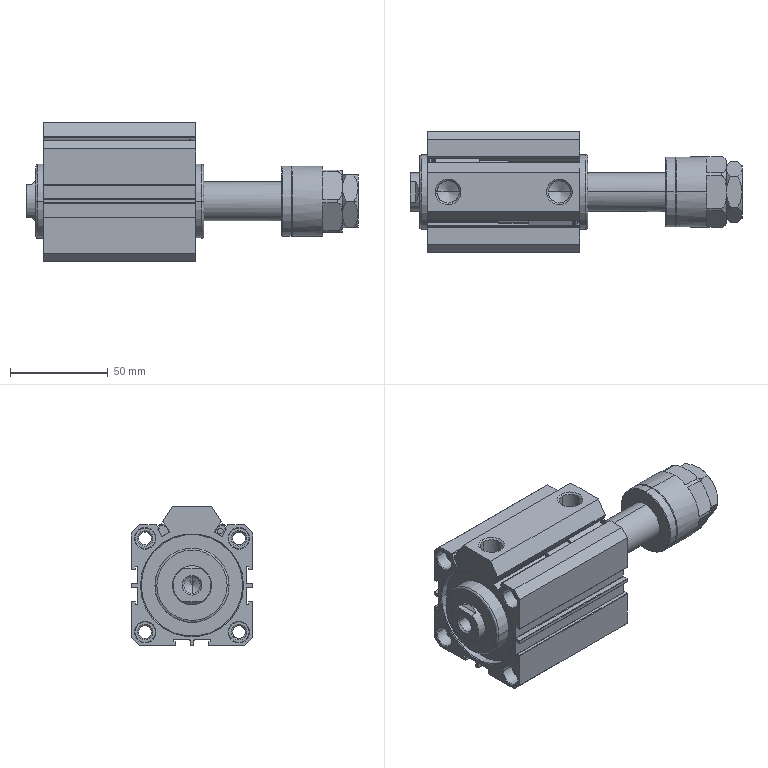Part | SolidWorks | features BaseBody 6 | 6 solids | 418 faces | box 170 x 62 x 71.5 mm | volume 267417 mm3 | plane 161 | cylinder 156 | cone 95 | spline 6 | commonest cylinder face diameters 0.4 x50 6.647 x16 10.5 x16 0.8 x10 6.5 x8 20 x8